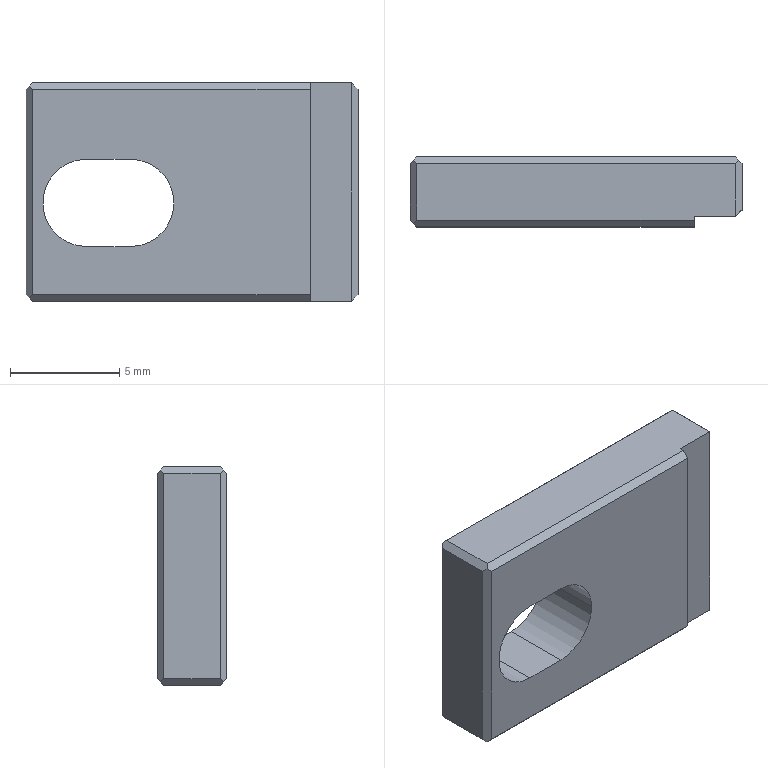Part | NX | 1 solid | 25 faces | box 15.2 x 3.2 x 10 mm | volume 405.331 mm3 | plane 22 | cylinder 3 | commonest cylinder face diameters 4 x3
STEP:
#1=CARTESIAN_POINT('',(1982.9,167.32,-119.));
#2=VERTEX_POINT('',#1);
#3=CARTESIAN_POINT('',(1982.9,167.32,-109.6));
#4=VERTEX_POINT('',#3);
#5=CARTESIAN_POINT('',(1982.9,167.32,-114.3));
#6=DIRECTION('',(0.,0.,1.));
#7=VECTOR('',#6,1000.);
#8=LINE('',#5,#7);
#9=EDGE_CURVE('',#2,#4,#8,.T.);
#10=ORIENTED_EDGE('',*,*,#9,.T.);
#11=CARTESIAN_POINT('',(1997.5,167.32,-109.6));
#12=VERTEX_POINT('',#11);
#13=CARTESIAN_POINT('',(1990.2,167.32,-109.6));
#14=DIRECTION('',(1.,0.,0.));
#15=VECTOR('',#14,1000.);
#16=LINE('',#13,#15);
#17=EDGE_CURVE('',#4,#12,#16,.T.);
#18=ORIENTED_EDGE('',*,*,#17,.T.);
#19=CARTESIAN_POINT('',(1997.5,167.32,-119.));
#20=VERTEX_POINT('',#19);
#21=CARTESIAN_POINT('',(1997.5,167.32,-114.3));
#22=DIRECTION('',(0.,0.,1.));
#23=VECTOR('',#22,1000.);
#24=LINE('',#21,#23);
#25=EDGE_CURVE('',#20,#12,#24,.T.);
#26=ORIENTED_EDGE('',*,*,#25,.F.);
#27=CARTESIAN_POINT('',(1990.2,167.32,-119.));
#28=DIRECTION('',(1.,0.,0.));
#29=VECTOR('',#28,1000.);
#30=LINE('',#27,#29);
#31=EDGE_CURVE('',#2,#20,#30,.T.);
#32=ORIENTED_EDGE('',*,*,#31,.F.);
#33=EDGE_LOOP('',(#10,#18,#26,#32));
#34=FACE_BOUND('',#33,.T.);
#35=CARTESIAN_POINT('',(1987.373,167.32,-112.8));
#36=VERTEX_POINT('',#35);
#37=CARTESIAN_POINT('',(1985.373,167.32,-112.8));
#38=VERTEX_POINT('',#37);
#39=CARTESIAN_POINT('',(1997.8,167.32,-112.8));
#40=DIRECTION('',(-1.,0.,0.));
#41=VECTOR('',#40,1000.);
#42=LINE('',#39,#41);
#43=EDGE_CURVE('',#36,#38,#42,.T.);
#44=ORIENTED_EDGE('',*,*,#43,.T.);
#45=CARTESIAN_POINT('',(1985.373,167.32,-116.8));
#46=VERTEX_POINT('',#45);
#47=CARTESIAN_POINT('',(1985.373,167.32,-114.8));
#48=DIRECTION('',(0.,-1.,0.));
#49=DIRECTION('',(1.,0.,0.));
#50=AXIS2_PLACEMENT_3D('',#47,#48,#49);
#51=CIRCLE('',#50,2.);
#52=EDGE_CURVE('',#38,#46,#51,.T.);
#53=ORIENTED_EDGE('',*,*,#52,.T.);
#54=CARTESIAN_POINT('',(1987.373,167.32,-116.8));
#55=VERTEX_POINT('',#54);
#56=CARTESIAN_POINT('',(1997.8,167.32,-116.8));
#57=DIRECTION('',(1.,0.,0.));
#58=VECTOR('',#57,1000.);
#59=LINE('',#56,#58);
#60=EDGE_CURVE('',#46,#55,#59,.T.);
#61=ORIENTED_EDGE('',*,*,#60,.T.);
#62=CARTESIAN_POINT('',(1989.373,167.32,-114.8));
#63=VERTEX_POINT('',#62);
#64=CARTESIAN_POINT('',(1987.373,167.32,-114.8));
#65=DIRECTION('',(0.,-1.,0.));
#66=DIRECTION('',(1.,0.,0.));
#67=AXIS2_PLACEMENT_3D('',#64,#65,#66);
#68=CIRCLE('',#67,2.);
#69=EDGE_CURVE('',#55,#63,#68,.T.);
#70=ORIENTED_EDGE('',*,*,#69,.T.);
#71=CARTESIAN_POINT('',(1987.373,167.32,-114.8));
#72=DIRECTION('',(0.,-1.,0.));
#73=DIRECTION('',(1.,0.,0.));
#74=AXIS2_PLACEMENT_3D('',#71,#72,#73);
#75=CIRCLE('',#74,2.);
#76=EDGE_CURVE('',#63,#36,#75,.T.);
#77=ORIENTED_EDGE('',*,*,#76,.T.);
#78=EDGE_LOOP('',(#44,#53,#61,#70,#77));
#79=FACE_BOUND('',#78,.T.);
#80=CARTESIAN_POINT('',(1997.8,167.32,-119.3));
#81=DIRECTION('',(0.,-1.,0.));
#82=DIRECTION('',(0.,0.,-1.));
#83=AXIS2_PLACEMENT_3D('',#80,#81,#82);
#84=PLANE('',#83);
#85=ADVANCED_FACE('',(#34,#79),#84,.F.);
#86=CARTESIAN_POINT('',(1997.8,164.9,-109.6));
#87=VERTEX_POINT('',#86);
#88=CARTESIAN_POINT('',(1997.8,164.9,-119.));
#89=VERTEX_POINT('',#88);
#90=CARTESIAN_POINT('',(1997.8,164.9,-114.3));
#91=DIRECTION('',(0.,0.,-1.));
#92=VECTOR('',#91,1000.);
#93=LINE('',#90,#92);
#94=EDGE_CURVE('',#87,#89,#93,.T.);
#95=ORIENTED_EDGE('',*,*,#94,.T.);
#96=CARTESIAN_POINT('',(1997.8,167.02,-119.));
#97=VERTEX_POINT('',#96);
#98=CARTESIAN_POINT('',(1997.8,165.96,-119.));
#99=DIRECTION('',(0.,-1.,0.));
#100=VECTOR('',#99,1000.);
#101=LINE('',#98,#100);
#102=EDGE_CURVE('',#97,#89,#101,.T.);
#103=ORIENTED_EDGE('',*,*,#102,.F.);
#104=CARTESIAN_POINT('',(1997.8,167.02,-109.6));
#105=VERTEX_POINT('',#104);
#106=CARTESIAN_POINT('',(1997.8,167.02,-114.3));
#107=DIRECTION('',(0.,0.,1.));
#108=VECTOR('',#107,1000.);
#109=LINE('',#106,#108);
#110=EDGE_CURVE('',#97,#105,#109,.T.);
#111=ORIENTED_EDGE('',*,*,#110,.T.);
#112=CARTESIAN_POINT('',(1997.8,165.96,-109.6));
#113=DIRECTION('',(0.,-1.,0.));
#114=VECTOR('',#113,1000.);
#115=LINE('',#112,#114);
#116=EDGE_CURVE('',#105,#87,#115,.T.);
#117=ORIENTED_EDGE('',*,*,#116,.T.);
#118=EDGE_LOOP('',(#95,#103,#111,#117));
#119=FACE_BOUND('',#118,.T.);
#120=CARTESIAN_POINT('',(1997.8,164.12,-119.3));
#121=DIRECTION('',(-1.,0.,0.));
#122=DIRECTION('',(0.,0.,1.));
#123=AXIS2_PLACEMENT_3D('',#120,#121,#122);
#124=PLANE('',#123);
#125=ADVANCED_FACE('',(#119),#124,.F.);
#126=CARTESIAN_POINT('',(1995.607,164.12,-109.6));
#127=VERTEX_POINT('',#126);
#128=CARTESIAN_POINT('',(1995.607,164.12,-119.));
#129=VERTEX_POINT('',#128);
#130=CARTESIAN_POINT('',(1995.607,164.12,-119.3));
#131=DIRECTION('',(0.,0.,-1.));
#132=VECTOR('',#131,1000.);
#133=LINE('',#130,#132);
#134=EDGE_CURVE('',#127,#129,#133,.T.);
#135=ORIENTED_EDGE('',*,*,#134,.F.);
#136=CARTESIAN_POINT('',(1982.9,164.12,-109.6));
#137=VERTEX_POINT('',#136);
#138=CARTESIAN_POINT('',(1989.104,164.12,-109.6));
#139=DIRECTION('',(-1.,0.,0.));
#140=VECTOR('',#139,1000.);
#141=LINE('',#138,#140);
#142=EDGE_CURVE('',#127,#137,#141,.T.);
#143=ORIENTED_EDGE('',*,*,#142,.T.);
#144=CARTESIAN_POINT('',(1982.9,164.12,-119.));
#145=VERTEX_POINT('',#144);
#146=CARTESIAN_POINT('',(1982.9,164.12,-114.3));
#147=DIRECTION('',(0.,0.,1.));
#148=VECTOR('',#147,1000.);
#149=LINE('',#146,#148);
#150=EDGE_CURVE('',#145,#137,#149,.T.);
#151=ORIENTED_EDGE('',*,*,#150,.F.);
#152=CARTESIAN_POINT('',(1989.104,164.12,-119.));
#153=DIRECTION('',(-1.,0.,0.));
#154=VECTOR('',#153,1000.);
#155=LINE('',#152,#154);
#156=EDGE_CURVE('',#129,#145,#155,.T.);
#157=ORIENTED_EDGE('',*,*,#156,.F.);
#158=EDGE_LOOP('',(#135,#143,#151,#157));
#159=FACE_BOUND('',#158,.T.);
#160=CARTESIAN_POINT('',(1987.373,164.12,-116.8));
#161=VERTEX_POINT('',#160);
#162=CARTESIAN_POINT('',(1989.373,164.12,-114.8));
#163=VERTEX_POINT('',#162);
#164=CARTESIAN_POINT('',(1987.373,164.12,-114.8));
#165=DIRECTION('',(0.,-1.,0.));
#166=DIRECTION('',(1.,0.,0.));
#167=AXIS2_PLACEMENT_3D('',#164,#165,#166);
#168=CIRCLE('',#167,2.);
#169=EDGE_CURVE('',#161,#163,#168,.T.);
#170=ORIENTED_EDGE('',*,*,#169,.F.);
#171=CARTESIAN_POINT('',(1985.373,164.12,-116.8));
#172=VERTEX_POINT('',#171);
#173=CARTESIAN_POINT('',(1997.8,164.12,-116.8));
#174=DIRECTION('',(-1.,0.,0.));
#175=VECTOR('',#174,1000.);
#176=LINE('',#173,#175);
#177=EDGE_CURVE('',#161,#172,#176,.T.);
#178=ORIENTED_EDGE('',*,*,#177,.T.);
#179=CARTESIAN_POINT('',(1985.373,164.12,-112.8));
#180=VERTEX_POINT('',#179);
#181=CARTESIAN_POINT('',(1985.373,164.12,-114.8));
#182=DIRECTION('',(0.,-1.,0.));
#183=DIRECTION('',(1.,0.,0.));
#184=AXIS2_PLACEMENT_3D('',#181,#182,#183);
#185=CIRCLE('',#184,2.);
#186=EDGE_CURVE('',#180,#172,#185,.T.);
#187=ORIENTED_EDGE('',*,*,#186,.F.);
#188=CARTESIAN_POINT('',(1987.373,164.12,-112.8));
#189=VERTEX_POINT('',#188);
#190=CARTESIAN_POINT('',(1997.8,164.12,-112.8));
#191=DIRECTION('',(1.,0.,0.));
#192=VECTOR('',#191,1000.);
#193=LINE('',#190,#192);
#194=EDGE_CURVE('',#180,#189,#193,.T.);
#195=ORIENTED_EDGE('',*,*,#194,.T.);
#196=CARTESIAN_POINT('',(1987.373,164.12,-114.8));
#197=DIRECTION('',(0.,-1.,0.));
#198=DIRECTION('',(1.,0.,0.));
#199=AXIS2_PLACEMENT_3D('',#196,#197,#198);
#200=CIRCLE('',#199,2.);
#201=EDGE_CURVE('',#163,#189,#200,.T.);
#202=ORIENTED_EDGE('',*,*,#201,.F.);
#203=EDGE_LOOP('',(#170,#178,#187,#195,#202));
#204=FACE_BOUND('',#203,.T.);
#205=CARTESIAN_POINT('',(1982.6,164.12,-119.3));
#206=DIRECTION('',(0.,1.,0.));
#207=DIRECTION('',(1.,0.,0.));
#208=AXIS2_PLACEMENT_3D('',#205,#206,#207);
#209=PLANE('',#208);
#210=ADVANCED_FACE('',(#159,#204),#209,.F.);
#211=CARTESIAN_POINT('',(1982.6,164.42,-119.));
#212=VERTEX_POINT('',#211);
#213=CARTESIAN_POINT('',(1982.6,164.42,-109.6));
#214=VERTEX_POINT('',#213);
#215=CARTESIAN_POINT('',(1982.6,164.42,-114.3));
#216=DIRECTION('',(0.,0.,1.));
#217=VECTOR('',#216,1000.);
#218=LINE('',#215,#217);
#219=EDGE_CURVE('',#212,#214,#218,.T.);
#220=ORIENTED_EDGE('',*,*,#219,.T.);
#221=CARTESIAN_POINT('',(1982.6,167.02,-109.6));
#222=VERTEX_POINT('',#221);
#223=CARTESIAN_POINT('',(1982.6,165.72,-109.6));
#224=DIRECTION('',(0.,1.,0.));
#225=VECTOR('',#224,1000.);
#226=LINE('',#223,#225);
#227=EDGE_CURVE('',#214,#222,#226,.T.);
#228=ORIENTED_EDGE('',*,*,#227,.T.);
#229=CARTESIAN_POINT('',(1982.6,167.02,-119.));
#230=VERTEX_POINT('',#229);
#231=CARTESIAN_POINT('',(1982.6,167.02,-114.3));
#232=DIRECTION('',(0.,0.,1.));
#233=VECTOR('',#232,1000.);
#234=LINE('',#231,#233);
#235=EDGE_CURVE('',#230,#222,#234,.T.);
#236=ORIENTED_EDGE('',*,*,#235,.F.);
#237=CARTESIAN_POINT('',(1982.6,165.72,-119.));
#238=DIRECTION('',(0.,1.,0.));
#239=VECTOR('',#238,1000.);
#240=LINE('',#237,#239);
#241=EDGE_CURVE('',#212,#230,#240,.T.);
#242=ORIENTED_EDGE('',*,*,#241,.F.);
#243=EDGE_LOOP('',(#220,#228,#236,#242));
#244=FACE_BOUND('',#243,.T.);
#245=CARTESIAN_POINT('',(1982.6,167.32,-119.3));
#246=DIRECTION('',(1.,0.,0.));
#247=DIRECTION('',(0.,1.,0.));
#248=AXIS2_PLACEMENT_3D('',#245,#246,#247);
#249=PLANE('',#248);
#250=ADVANCED_FACE('',(#244),#249,.F.);
#251=ORIENTED_EDGE('',*,*,#186,.T.);
#252=CARTESIAN_POINT('',(1985.373,163.8,-116.8));
#253=DIRECTION('',(0.,1.,0.));
#254=VECTOR('',#253,1000.);
#255=LINE('',#252,#254);
#256=EDGE_CURVE('',#172,#46,#255,.T.);
#257=ORIENTED_EDGE('',*,*,#256,.T.);
#258=ORIENTED_EDGE('',*,*,#52,.F.);
#259=CARTESIAN_POINT('',(1985.373,163.8,-112.8));
#260=DIRECTION('',(0.,1.,0.));
#261=VECTOR('',#260,1000.);
#262=LINE('',#259,#261);
#263=EDGE_CURVE('',#180,#38,#262,.T.);
#264=ORIENTED_EDGE('',*,*,#263,.F.);
#265=EDGE_LOOP('',(#251,#257,#258,#264));
#266=FACE_BOUND('',#265,.T.);
#267=CARTESIAN_POINT('',(1985.373,163.8,-114.8));
#268=DIRECTION('',(0.,-1.,0.));
#269=DIRECTION('',(1.,0.,0.));
#270=AXIS2_PLACEMENT_3D('',#267,#268,#269);
#271=CYLINDRICAL_SURFACE('',#270,2.);
#272=ADVANCED_FACE('',(#266),#271,.F.);
#273=ORIENTED_EDGE('',*,*,#177,.F.);
#274=CARTESIAN_POINT('',(1987.373,163.8,-116.8));
#275=DIRECTION('',(0.,1.,0.));
#276=VECTOR('',#275,1000.);
#277=LINE('',#274,#276);
#278=EDGE_CURVE('',#161,#55,#277,.T.);
#279=ORIENTED_EDGE('',*,*,#278,.T.);
#280=ORIENTED_EDGE('',*,*,#60,.F.);
#281=ORIENTED_EDGE('',*,*,#256,.F.);
#282=EDGE_LOOP('',(#273,#279,#280,#281));
#283=FACE_BOUND('',#282,.T.);
#284=CARTESIAN_POINT('',(1985.373,163.8,-116.8));
#285=DIRECTION('',(0.,0.,-1.));
#286=DIRECTION('',(0.,-1.,0.));
#287=AXIS2_PLACEMENT_3D('',#284,#285,#286);
#288=PLANE('',#287);
#289=ADVANCED_FACE('',(#283),#288,.F.);
#290=CARTESIAN_POINT('',(1989.373,163.8,-114.8));
#291=DIRECTION('',(0.,-1.,0.));
#292=VECTOR('',#291,1000.);
#293=LINE('',#290,#292);
#294=EDGE_CURVE('',#63,#163,#293,.T.);
#295=ORIENTED_EDGE('',*,*,#294,.F.);
#296=ORIENTED_EDGE('',*,*,#69,.F.);
#297=ORIENTED_EDGE('',*,*,#278,.F.);
#298=ORIENTED_EDGE('',*,*,#169,.T.);
#299=EDGE_LOOP('',(#295,#296,#297,#298));
#300=FACE_BOUND('',#299,.T.);
#301=CARTESIAN_POINT('',(1987.373,163.8,-114.8));
#302=DIRECTION('',(0.,-1.,0.));
#303=DIRECTION('',(1.,0.,0.));
#304=AXIS2_PLACEMENT_3D('',#301,#302,#303);
#305=CYLINDRICAL_SURFACE('',#304,2.);
#306=ADVANCED_FACE('',(#300),#305,.F.);
#307=ORIENTED_EDGE('',*,*,#194,.F.);
#308=ORIENTED_EDGE('',*,*,#263,.T.);
#309=ORIENTED_EDGE('',*,*,#43,.F.);
#310=CARTESIAN_POINT('',(1987.373,163.8,-112.8));
#311=DIRECTION('',(0.,1.,0.));
#312=VECTOR('',#311,1000.);
#313=LINE('',#310,#312);
#314=EDGE_CURVE('',#189,#36,#313,.T.);
#315=ORIENTED_EDGE('',*,*,#314,.F.);
#316=EDGE_LOOP('',(#307,#308,#309,#315));
#317=FACE_BOUND('',#316,.T.);
#318=CARTESIAN_POINT('',(1987.373,163.8,-112.8));
#319=DIRECTION('',(0.,0.,1.));
#320=DIRECTION('',(1.,0.,0.));
#321=AXIS2_PLACEMENT_3D('',#318,#319,#320);
#322=PLANE('',#321);
#323=ADVANCED_FACE('',(#317),#322,.F.);
#324=ORIENTED_EDGE('',*,*,#25,.T.);
#325=CARTESIAN_POINT('',(1997.65,167.17,-109.45));
#326=VERTEX_POINT('',#325);
#327=CARTESIAN_POINT('',(1987.8,177.02,-119.3));
#328=DIRECTION('',(0.5774,-0.5774,0.5774));
#329=VECTOR('',#328,1000.);
#330=LINE('',#327,#329);
#331=EDGE_CURVE('',#12,#326,#330,.T.);
#332=ORIENTED_EDGE('',*,*,#331,.T.);
#333=CARTESIAN_POINT('',(2007.5,157.32,-119.3));
#334=DIRECTION('',(0.5774,-0.5774,-0.5774));
#335=VECTOR('',#334,1000.);
#336=LINE('',#333,#335);
#337=EDGE_CURVE('',#326,#105,#336,.T.);
#338=ORIENTED_EDGE('',*,*,#337,.T.);
#339=ORIENTED_EDGE('',*,*,#110,.F.);
#340=CARTESIAN_POINT('',(1997.65,167.17,-119.15));
#341=VERTEX_POINT('',#340);
#342=CARTESIAN_POINT('',(2016.57,148.25,-100.23));
#343=DIRECTION('',(0.5774,-0.5774,0.5774));
#344=VECTOR('',#343,1000.);
#345=LINE('',#342,#344);
#346=EDGE_CURVE('',#341,#97,#345,.T.);
#347=ORIENTED_EDGE('',*,*,#346,.F.);
#348=CARTESIAN_POINT('',(2016.57,148.25,-138.07));
#349=DIRECTION('',(0.5774,-0.5774,-0.5774));
#350=VECTOR('',#349,1000.);
#351=LINE('',#348,#350);
#352=EDGE_CURVE('',#20,#341,#351,.T.);
#353=ORIENTED_EDGE('',*,*,#352,.F.);
#354=EDGE_LOOP('',(#324,#332,#338,#339,#347,#353));
#355=FACE_BOUND('',#354,.T.);
#356=CARTESIAN_POINT('',(1997.65,167.17,-114.3));
#357=DIRECTION('',(-0.7071,-0.7071,0.));
#358=DIRECTION('',(-0.7071,0.7071,0.));
#359=AXIS2_PLACEMENT_3D('',#356,#357,#358);
#360=PLANE('',#359);
#361=ADVANCED_FACE('',(#355),#360,.F.);
#362=ORIENTED_EDGE('',*,*,#94,.F.);
#363=CARTESIAN_POINT('',(1997.5,164.6,-109.3));
#364=VERTEX_POINT('',#363);
#365=CARTESIAN_POINT('',(2007.5,174.6,-119.3));
#366=DIRECTION('',(-0.5774,-0.5774,0.5774));
#367=VECTOR('',#366,1000.);
#368=LINE('',#365,#367);
#369=EDGE_CURVE('',#87,#364,#368,.T.);
#370=ORIENTED_EDGE('',*,*,#369,.T.);
#371=CARTESIAN_POINT('',(1997.5,164.6,-119.3));
#372=VERTEX_POINT('',#371);
#373=CARTESIAN_POINT('',(1997.5,164.6,-114.3));
#374=DIRECTION('',(0.,0.,-1.));
#375=VECTOR('',#374,1000.);
#376=LINE('',#373,#375);
#377=EDGE_CURVE('',#364,#372,#376,.T.);
#378=ORIENTED_EDGE('',*,*,#377,.T.);
#379=CARTESIAN_POINT('',(1981.15,148.25,-135.65));
#380=DIRECTION('',(0.5774,0.5774,0.5774));
#381=VECTOR('',#380,1000.);
#382=LINE('',#379,#381);
#383=EDGE_CURVE('',#372,#89,#382,.T.);
#384=ORIENTED_EDGE('',*,*,#383,.T.);
#385=EDGE_LOOP('',(#362,#370,#378,#384));
#386=FACE_BOUND('',#385,.T.);
#387=CARTESIAN_POINT('',(1997.65,164.75,-114.3));
#388=DIRECTION('',(0.7071,-0.7071,0.));
#389=DIRECTION('',(0.,0.,-1.));
#390=AXIS2_PLACEMENT_3D('',#387,#388,#389);
#391=PLANE('',#390);
#392=ADVANCED_FACE('',(#386),#391,.T.);
#393=ORIENTED_EDGE('',*,*,#9,.F.);
#394=CARTESIAN_POINT('',(1982.75,167.17,-119.15));
#395=VERTEX_POINT('',#394);
#396=CARTESIAN_POINT('',(1997.8,182.22,-104.1));
#397=DIRECTION('',(-0.5774,-0.5774,-0.5774));
#398=VECTOR('',#397,1000.);
#399=LINE('',#396,#398);
#400=EDGE_CURVE('',#2,#395,#399,.T.);
#401=ORIENTED_EDGE('',*,*,#400,.T.);
#402=CARTESIAN_POINT('',(1997.8,182.22,-134.2));
#403=DIRECTION('',(-0.5774,-0.5774,0.5774));
#404=VECTOR('',#403,1000.);
#405=LINE('',#402,#404);
#406=EDGE_CURVE('',#395,#230,#405,.T.);
#407=ORIENTED_EDGE('',*,*,#406,.T.);
#408=ORIENTED_EDGE('',*,*,#235,.T.);
#409=CARTESIAN_POINT('',(1982.75,167.17,-109.45));
#410=VERTEX_POINT('',#409);
#411=CARTESIAN_POINT('',(1972.9,157.32,-119.3));
#412=DIRECTION('',(0.5774,0.5774,0.5774));
#413=VECTOR('',#412,1000.);
#414=LINE('',#411,#413);
#415=EDGE_CURVE('',#222,#410,#414,.T.);
#416=ORIENTED_EDGE('',*,*,#415,.T.);
#417=CARTESIAN_POINT('',(1992.6,177.02,-119.3));
#418=DIRECTION('',(0.5774,0.5774,-0.5774));
#419=VECTOR('',#418,1000.);
#420=LINE('',#417,#419);
#421=EDGE_CURVE('',#410,#4,#420,.T.);
#422=ORIENTED_EDGE('',*,*,#421,.T.);
#423=EDGE_LOOP('',(#393,#401,#407,#408,#416,#422));
#424=FACE_BOUND('',#423,.T.);
#425=CARTESIAN_POINT('',(1982.75,167.17,-114.3));
#426=DIRECTION('',(-0.7071,0.7071,0.));
#427=DIRECTION('',(0.,0.,1.));
#428=AXIS2_PLACEMENT_3D('',#425,#426,#427);
#429=PLANE('',#428);
#430=ADVANCED_FACE('',(#424),#429,.T.);
#431=ORIENTED_EDGE('',*,*,#219,.F.);
#432=CARTESIAN_POINT('',(1982.75,164.27,-119.15));
#433=VERTEX_POINT('',#432);
#434=CARTESIAN_POINT('',(1997.8,149.22,-134.2));
#435=DIRECTION('',(0.5774,-0.5774,-0.5774));
#436=VECTOR('',#435,1000.);
#437=LINE('',#434,#436);
#438=EDGE_CURVE('',#212,#433,#437,.T.);
#439=ORIENTED_EDGE('',*,*,#438,.T.);
#440=CARTESIAN_POINT('',(1997.8,149.22,-104.1));
#441=DIRECTION('',(0.5774,-0.5774,0.5774));
#442=VECTOR('',#441,1000.);
#443=LINE('',#440,#442);
#444=EDGE_CURVE('',#433,#145,#443,.T.);
#445=ORIENTED_EDGE('',*,*,#444,.T.);
#446=ORIENTED_EDGE('',*,*,#150,.T.);
#447=CARTESIAN_POINT('',(1982.75,164.27,-109.45));
#448=VERTEX_POINT('',#447);
#449=CARTESIAN_POINT('',(1992.6,154.42,-119.3));
#450=DIRECTION('',(-0.5774,0.5774,0.5774));
#451=VECTOR('',#450,1000.);
#452=LINE('',#449,#451);
#453=EDGE_CURVE('',#137,#448,#452,.T.);
#454=ORIENTED_EDGE('',*,*,#453,.T.);
#455=CARTESIAN_POINT('',(1972.9,174.12,-119.3));
#456=DIRECTION('',(-0.5774,0.5774,-0.5774));
#457=VECTOR('',#456,1000.);
#458=LINE('',#455,#457);
#459=EDGE_CURVE('',#448,#214,#458,.T.);
#460=ORIENTED_EDGE('',*,*,#459,.T.);
#461=EDGE_LOOP('',(#431,#439,#445,#446,#454,#460));
#462=FACE_BOUND('',#461,.T.);
#463=CARTESIAN_POINT('',(1982.75,164.27,-114.3));
#464=DIRECTION('',(-0.7071,-0.7071,0.));
#465=DIRECTION('',(-0.7071,0.7071,0.));
#466=AXIS2_PLACEMENT_3D('',#463,#464,#465);
#467=PLANE('',#466);
#468=ADVANCED_FACE('',(#462),#467,.T.);
#469=CARTESIAN_POINT('',(1982.9,164.42,-109.3));
#470=VERTEX_POINT('',#469);
#471=CARTESIAN_POINT('',(1982.9,167.02,-109.3));
#472=VERTEX_POINT('',#471);
#473=CARTESIAN_POINT('',(1982.9,165.72,-109.3));
#474=DIRECTION('',(0.,1.,0.));
#475=VECTOR('',#474,1000.);
#476=LINE('',#473,#475);
#477=EDGE_CURVE('',#470,#472,#476,.T.);
#478=ORIENTED_EDGE('',*,*,#477,.F.);
#479=CARTESIAN_POINT('',(1995.607,164.42,-109.3));
#480=VERTEX_POINT('',#479);
#481=CARTESIAN_POINT('',(1989.104,164.42,-109.3));
#482=DIRECTION('',(-1.,0.,0.));
#483=VECTOR('',#482,1000.);
#484=LINE('',#481,#483);
#485=EDGE_CURVE('',#480,#470,#484,.T.);
#486=ORIENTED_EDGE('',*,*,#485,.F.);
#487=CARTESIAN_POINT('',(1995.607,164.6,-109.3));
#488=VERTEX_POINT('',#487);
#489=CARTESIAN_POINT('',(1995.607,148.25,-109.3));
#490=DIRECTION('',(0.,-1.,0.));
#491=VECTOR('',#490,1000.);
#492=LINE('',#489,#491);
#493=EDGE_CURVE('',#488,#480,#492,.T.);
#494=ORIENTED_EDGE('',*,*,#493,.F.);
#495=CARTESIAN_POINT('',(1997.8,164.6,-109.3));
#496=DIRECTION('',(1.,0.,0.));
#497=VECTOR('',#496,1000.);
#498=LINE('',#495,#497);
#499=EDGE_CURVE('',#488,#364,#498,.T.);
#500=ORIENTED_EDGE('',*,*,#499,.T.);
#501=CARTESIAN_POINT('',(1997.5,167.02,-109.3));
#502=VERTEX_POINT('',#501);
#503=CARTESIAN_POINT('',(1997.5,165.96,-109.3));
#504=DIRECTION('',(0.,-1.,0.));
#505=VECTOR('',#504,1000.);
#506=LINE('',#503,#505);
#507=EDGE_CURVE('',#502,#364,#506,.T.);
#508=ORIENTED_EDGE('',*,*,#507,.F.);
#509=CARTESIAN_POINT('',(1990.2,167.02,-109.3));
#510=DIRECTION('',(1.,0.,0.));
#511=VECTOR('',#510,1000.);
#512=LINE('',#509,#511);
#513=EDGE_CURVE('',#472,#502,#512,.T.);
#514=ORIENTED_EDGE('',*,*,#513,.F.);
#515=EDGE_LOOP('',(#478,#486,#494,#500,#508,#514));
#516=FACE_BOUND('',#515,.T.);
#517=CARTESIAN_POINT('',(1997.8,148.25,-109.3));
#518=DIRECTION('',(0.,0.,-1.));
#519=DIRECTION('',(0.,-1.,0.));
#520=AXIS2_PLACEMENT_3D('',#517,#518,#519);
#521=PLANE('',#520);
#522=ADVANCED_FACE('',(#516),#521,.F.);
#523=ORIENTED_EDGE('',*,*,#513,.T.);
#524=CARTESIAN_POINT('',(2007.5,177.02,-119.3));
#525=DIRECTION('',(0.5774,0.5774,-0.5774));
#526=VECTOR('',#525,1000.);
#527=LINE('',#524,#526);
#528=EDGE_CURVE('',#502,#326,#527,.T.);
#529=ORIENTED_EDGE('',*,*,#528,.T.);
#530=ORIENTED_EDGE('',*,*,#331,.F.);
#531=ORIENTED_EDGE('',*,*,#17,.F.);
#532=ORIENTED_EDGE('',*,*,#421,.F.);
#533=CARTESIAN_POINT('',(1972.9,177.02,-119.3));
#534=DIRECTION('',(0.5774,-0.5774,0.5774));
#535=VECTOR('',#534,1000.);
#536=LINE('',#533,#535);
#537=EDGE_CURVE('',#410,#472,#536,.T.);
#538=ORIENTED_EDGE('',*,*,#537,.T.);
#539=EDGE_LOOP('',(#523,#529,#530,#531,#532,#538));
#540=FACE_BOUND('',#539,.T.);
#541=CARTESIAN_POINT('',(1990.2,167.17,-109.45));
#542=DIRECTION('',(0.,-0.7071,-0.7071));
#543=DIRECTION('',(0.,-0.7071,0.7071));
#544=AXIS2_PLACEMENT_3D('',#541,#542,#543);
#545=PLANE('',#544);
#546=ADVANCED_FACE('',(#540),#545,.F.);
#547=ORIENTED_EDGE('',*,*,#507,.T.);
#548=ORIENTED_EDGE('',*,*,#369,.F.);
#549=ORIENTED_EDGE('',*,*,#116,.F.);
#550=ORIENTED_EDGE('',*,*,#337,.F.);
#551=ORIENTED_EDGE('',*,*,#528,.F.);
#552=EDGE_LOOP('',(#547,#548,#549,#550,#551));
#553=FACE_BOUND('',#552,.T.);
#554=CARTESIAN_POINT('',(1997.65,165.96,-109.45));
#555=DIRECTION('',(-0.7071,0.,-0.7071));
#556=DIRECTION('',(-0.7071,0.,0.7071));
#557=AXIS2_PLACEMENT_3D('',#554,#555,#556);
#558=PLANE('',#557);
#559=ADVANCED_FACE('',(#553),#558,.F.);
#560=ORIENTED_EDGE('',*,*,#485,.T.);
#561=CARTESIAN_POINT('',(1972.9,154.42,-119.3));
#562=DIRECTION('',(-0.5774,-0.5774,-0.5774));
#563=VECTOR('',#562,1000.);
#564=LINE('',#561,#563);
#565=EDGE_CURVE('',#470,#448,#564,.T.);
#566=ORIENTED_EDGE('',*,*,#565,.T.);
#567=ORIENTED_EDGE('',*,*,#453,.F.);
#568=ORIENTED_EDGE('',*,*,#142,.F.);
#569=CARTESIAN_POINT('',(1995.607,154.42,-119.3));
#570=DIRECTION('',(0.,0.7071,0.7071));
#571=VECTOR('',#570,1000.);
#572=LINE('',#569,#571);
#573=EDGE_CURVE('',#127,#480,#572,.T.);
#574=ORIENTED_EDGE('',*,*,#573,.T.);
#575=EDGE_LOOP('',(#560,#566,#567,#568,#574));
#576=FACE_BOUND('',#575,.T.);
#577=CARTESIAN_POINT('',(1989.104,164.27,-109.45));
#578=DIRECTION('',(0.,0.7071,-0.7071));
#579=DIRECTION('',(-1.,0.,0.));
#580=AXIS2_PLACEMENT_3D('',#577,#578,#579);
#581=PLANE('',#580);
#582=ADVANCED_FACE('',(#576),#581,.F.);
#583=ORIENTED_EDGE('',*,*,#477,.T.);
#584=ORIENTED_EDGE('',*,*,#537,.F.);
#585=ORIENTED_EDGE('',*,*,#415,.F.);
#586=ORIENTED_EDGE('',*,*,#227,.F.);
#587=ORIENTED_EDGE('',*,*,#459,.F.);
#588=ORIENTED_EDGE('',*,*,#565,.F.);
#589=EDGE_LOOP('',(#583,#584,#585,#586,#587,#588));
#590=FACE_BOUND('',#589,.T.);
#591=CARTESIAN_POINT('',(1982.75,165.72,-109.45));
#592=DIRECTION('',(0.7071,0.,-0.7071));
#593=DIRECTION('',(0.,-1.,0.));
#594=AXIS2_PLACEMENT_3D('',#591,#592,#593);
#595=PLANE('',#594);
#596=ADVANCED_FACE('',(#590),#595,.F.);
#597=ORIENTED_EDGE('',*,*,#134,.T.);
#598=CARTESIAN_POINT('',(1995.607,164.42,-119.3));
#599=VERTEX_POINT('',#598);
#600=CARTESIAN_POINT('',(1995.607,148.25,-103.13));
#601=DIRECTION('',(0.,0.7071,-0.7071));
#602=VECTOR('',#601,1000.);
#603=LINE('',#600,#602);
#604=EDGE_CURVE('',#129,#599,#603,.T.);
#605=ORIENTED_EDGE('',*,*,#604,.T.);
#606=CARTESIAN_POINT('',(1995.607,164.6,-119.3));
#607=VERTEX_POINT('',#606);
#608=CARTESIAN_POINT('',(1995.607,148.25,-119.3));
#609=DIRECTION('',(0.,1.,0.));
#610=VECTOR('',#609,1000.);
#611=LINE('',#608,#610);
#612=EDGE_CURVE('',#599,#607,#611,.T.);
#613=ORIENTED_EDGE('',*,*,#612,.T.);
#614=CARTESIAN_POINT('',(1995.607,164.6,-120.3));
#615=DIRECTION('',(0.,0.,1.));
#616=VECTOR('',#615,1000.);
#617=LINE('',#614,#616);
#618=EDGE_CURVE('',#607,#488,#617,.T.);
#619=ORIENTED_EDGE('',*,*,#618,.T.);
#620=ORIENTED_EDGE('',*,*,#493,.T.);
#621=ORIENTED_EDGE('',*,*,#573,.F.);
#622=EDGE_LOOP('',(#597,#605,#613,#619,#620,#621));
#623=FACE_BOUND('',#622,.T.);
#624=CARTESIAN_POINT('',(1995.607,160.9,-120.3));
#625=DIRECTION('',(-1.,0.,0.));
#626=DIRECTION('',(0.,0.,1.));
#627=AXIS2_PLACEMENT_3D('',#624,#625,#626);
#628=PLANE('',#627);
#629=ADVANCED_FACE('',(#623),#628,.F.);
#630=CARTESIAN_POINT('',(1997.5,167.02,-119.3));
#631=VERTEX_POINT('',#630);
#632=CARTESIAN_POINT('',(1997.5,165.96,-119.3));
#633=DIRECTION('',(0.,-1.,0.));
#634=VECTOR('',#633,1000.);
#635=LINE('',#632,#634);
#636=EDGE_CURVE('',#631,#372,#635,.T.);
#637=ORIENTED_EDGE('',*,*,#636,.T.);
#638=CARTESIAN_POINT('',(1997.8,164.6,-119.3));
#639=DIRECTION('',(-1.,0.,0.));
#640=VECTOR('',#639,1000.);
#641=LINE('',#638,#640);
#642=EDGE_CURVE('',#372,#607,#641,.T.);
#643=ORIENTED_EDGE('',*,*,#642,.T.);
#644=ORIENTED_EDGE('',*,*,#612,.F.);
#645=CARTESIAN_POINT('',(1982.9,164.42,-119.3));
#646=VERTEX_POINT('',#645);
#647=CARTESIAN_POINT('',(1989.104,164.42,-119.3));
#648=DIRECTION('',(-1.,0.,0.));
#649=VECTOR('',#648,1000.);
#650=LINE('',#647,#649);
#651=EDGE_CURVE('',#599,#646,#650,.T.);
#652=ORIENTED_EDGE('',*,*,#651,.T.);
#653=CARTESIAN_POINT('',(1982.9,167.02,-119.3));
#654=VERTEX_POINT('',#653);
#655=CARTESIAN_POINT('',(1982.9,165.72,-119.3));
#656=DIRECTION('',(0.,1.,0.));
#657=VECTOR('',#656,1000.);
#658=LINE('',#655,#657);
#659=EDGE_CURVE('',#646,#654,#658,.T.);
#660=ORIENTED_EDGE('',*,*,#659,.T.);
#661=CARTESIAN_POINT('',(1990.2,167.02,-119.3));
#662=DIRECTION('',(1.,0.,0.));
#663=VECTOR('',#662,1000.);
#664=LINE('',#661,#663);
#665=EDGE_CURVE('',#654,#631,#664,.T.);
#666=ORIENTED_EDGE('',*,*,#665,.T.);
#667=EDGE_LOOP('',(#637,#643,#644,#652,#660,#666));
#668=FACE_BOUND('',#667,.T.);
#669=CARTESIAN_POINT('',(1997.8,148.25,-119.3));
#670=DIRECTION('',(0.,0.,-1.));
#671=DIRECTION('',(0.,-1.,0.));
#672=AXIS2_PLACEMENT_3D('',#669,#670,#671);
#673=PLANE('',#672);
#674=ADVANCED_FACE('',(#668),#673,.T.);
#675=ORIENTED_EDGE('',*,*,#377,.F.);
#676=ORIENTED_EDGE('',*,*,#499,.F.);
#677=ORIENTED_EDGE('',*,*,#618,.F.);
#678=ORIENTED_EDGE('',*,*,#642,.F.);
#679=EDGE_LOOP('',(#675,#676,#677,#678));
#680=FACE_BOUND('',#679,.T.);
#681=CARTESIAN_POINT('',(1996.107,164.6,-120.3));
#682=DIRECTION('',(0.,1.,0.));
#683=DIRECTION('',(1.,0.,0.));
#684=AXIS2_PLACEMENT_3D('',#681,#682,#683);
#685=PLANE('',#684);
#686=ADVANCED_FACE('',(#680),#685,.F.);
#687=ORIENTED_EDGE('',*,*,#659,.F.);
#688=CARTESIAN_POINT('',(1997.8,179.32,-134.2));
#689=DIRECTION('',(-0.5774,-0.5774,0.5774));
#690=VECTOR('',#689,1000.);
#691=LINE('',#688,#690);
#692=EDGE_CURVE('',#646,#433,#691,.T.);
#693=ORIENTED_EDGE('',*,*,#692,.T.);
#694=ORIENTED_EDGE('',*,*,#438,.F.);
#695=ORIENTED_EDGE('',*,*,#241,.T.);
#696=ORIENTED_EDGE('',*,*,#406,.F.);
#697=CARTESIAN_POINT('',(1997.8,152.12,-134.2));
#698=DIRECTION('',(0.5774,-0.5774,-0.5774));
#699=VECTOR('',#698,1000.);
#700=LINE('',#697,#699);
#701=EDGE_CURVE('',#395,#654,#700,.T.);
#702=ORIENTED_EDGE('',*,*,#701,.T.);
#703=EDGE_LOOP('',(#687,#693,#694,#695,#696,#702));
#704=FACE_BOUND('',#703,.T.);
#705=CARTESIAN_POINT('',(1982.75,165.72,-119.15));
#706=DIRECTION('',(-0.7071,0.,-0.7071));
#707=DIRECTION('',(-0.7071,0.,0.7071));
#708=AXIS2_PLACEMENT_3D('',#705,#706,#707);
#709=PLANE('',#708);
#710=ADVANCED_FACE('',(#704),#709,.T.);
#711=ORIENTED_EDGE('',*,*,#665,.F.);
#712=ORIENTED_EDGE('',*,*,#701,.F.);
#713=ORIENTED_EDGE('',*,*,#400,.F.);
#714=ORIENTED_EDGE('',*,*,#31,.T.);
#715=ORIENTED_EDGE('',*,*,#352,.T.);
#716=CARTESIAN_POINT('',(1978.73,148.25,-138.07));
#717=DIRECTION('',(-0.5774,-0.5774,-0.5774));
#718=VECTOR('',#717,1000.);
#719=LINE('',#716,#718);
#720=EDGE_CURVE('',#341,#631,#719,.T.);
#721=ORIENTED_EDGE('',*,*,#720,.T.);
#722=EDGE_LOOP('',(#711,#712,#713,#714,#715,#721));
#723=FACE_BOUND('',#722,.T.);
#724=CARTESIAN_POINT('',(1990.2,167.17,-119.15));
#725=DIRECTION('',(0.,0.7071,-0.7071));
#726=DIRECTION('',(-1.,0.,0.));
#727=AXIS2_PLACEMENT_3D('',#724,#725,#726);
#728=PLANE('',#727);
#729=ADVANCED_FACE('',(#723),#728,.T.);
#730=ORIENTED_EDGE('',*,*,#651,.F.);
#731=ORIENTED_EDGE('',*,*,#604,.F.);
#732=ORIENTED_EDGE('',*,*,#156,.T.);
#733=ORIENTED_EDGE('',*,*,#444,.F.);
#734=ORIENTED_EDGE('',*,*,#692,.F.);
#735=EDGE_LOOP('',(#730,#731,#732,#733,#734));
#736=FACE_BOUND('',#735,.T.);
#737=CARTESIAN_POINT('',(1989.104,164.27,-119.15));
#738=DIRECTION('',(0.,-0.7071,-0.7071));
#739=DIRECTION('',(0.,-0.7071,0.7071));
#740=AXIS2_PLACEMENT_3D('',#737,#738,#739);
#741=PLANE('',#740);
#742=ADVANCED_FACE('',(#736),#741,.T.);
#743=ORIENTED_EDGE('',*,*,#636,.F.);
#744=ORIENTED_EDGE('',*,*,#720,.F.);
#745=ORIENTED_EDGE('',*,*,#346,.T.);
#746=ORIENTED_EDGE('',*,*,#102,.T.);
#747=ORIENTED_EDGE('',*,*,#383,.F.);
#748=EDGE_LOOP('',(#743,#744,#745,#746,#747));
#749=FACE_BOUND('',#748,.T.);
#750=CARTESIAN_POINT('',(1997.65,165.96,-119.15));
#751=DIRECTION('',(0.7071,0.,-0.7071));
#752=DIRECTION('',(0.,-1.,0.));
#753=AXIS2_PLACEMENT_3D('',#750,#751,#752);
#754=PLANE('',#753);
#755=ADVANCED_FACE('',(#749),#754,.T.);
#756=ORIENTED_EDGE('',*,*,#76,.F.);
#757=ORIENTED_EDGE('',*,*,#294,.T.);
#758=ORIENTED_EDGE('',*,*,#201,.T.);
#759=ORIENTED_EDGE('',*,*,#314,.T.);
#760=EDGE_LOOP('',(#756,#757,#758,#759));
#761=FACE_BOUND('',#760,.T.);
#762=CARTESIAN_POINT('',(1987.373,163.8,-114.8));
#763=DIRECTION('',(0.,-1.,0.));
#764=DIRECTION('',(1.,0.,0.));
#765=AXIS2_PLACEMENT_3D('',#762,#763,#764);
#766=CYLINDRICAL_SURFACE('',#765,2.);
#767=ADVANCED_FACE('',(#761),#766,.F.);
#768=CLOSED_SHELL('',(#85,#125,#210,#250,#272,#289,#306,#323,#361,#392,#430,#468,#522,#546,#559,#582,#596,#629,#674,#686,#710,#729,#742,#755,#767));
#769=MANIFOLD_SOLID_BREP('',#768);
#770=(LENGTH_UNIT()NAMED_UNIT(*)SI_UNIT(.MILLI.,.METRE.));
#771=UNCERTAINTY_MEASURE_WITH_UNIT(LENGTH_MEASURE(0.00001),#770,'','');
#772=(NAMED_UNIT(*)PLANE_ANGLE_UNIT()SI_UNIT($,.RADIAN.));
#773=(NAMED_UNIT(*)SI_UNIT($,.STERADIAN.)SOLID_ANGLE_UNIT());
#774=(GEOMETRIC_REPRESENTATION_CONTEXT(3)GLOBAL_UNCERTAINTY_ASSIGNED_CONTEXT((#771))GLOBAL_UNIT_ASSIGNED_CONTEXT((#770,#772,#773))REPRESENTATION_CONTEXT('',''));
#775=ADVANCED_BREP_SHAPE_REPRESENTATION('',(#769),#774);